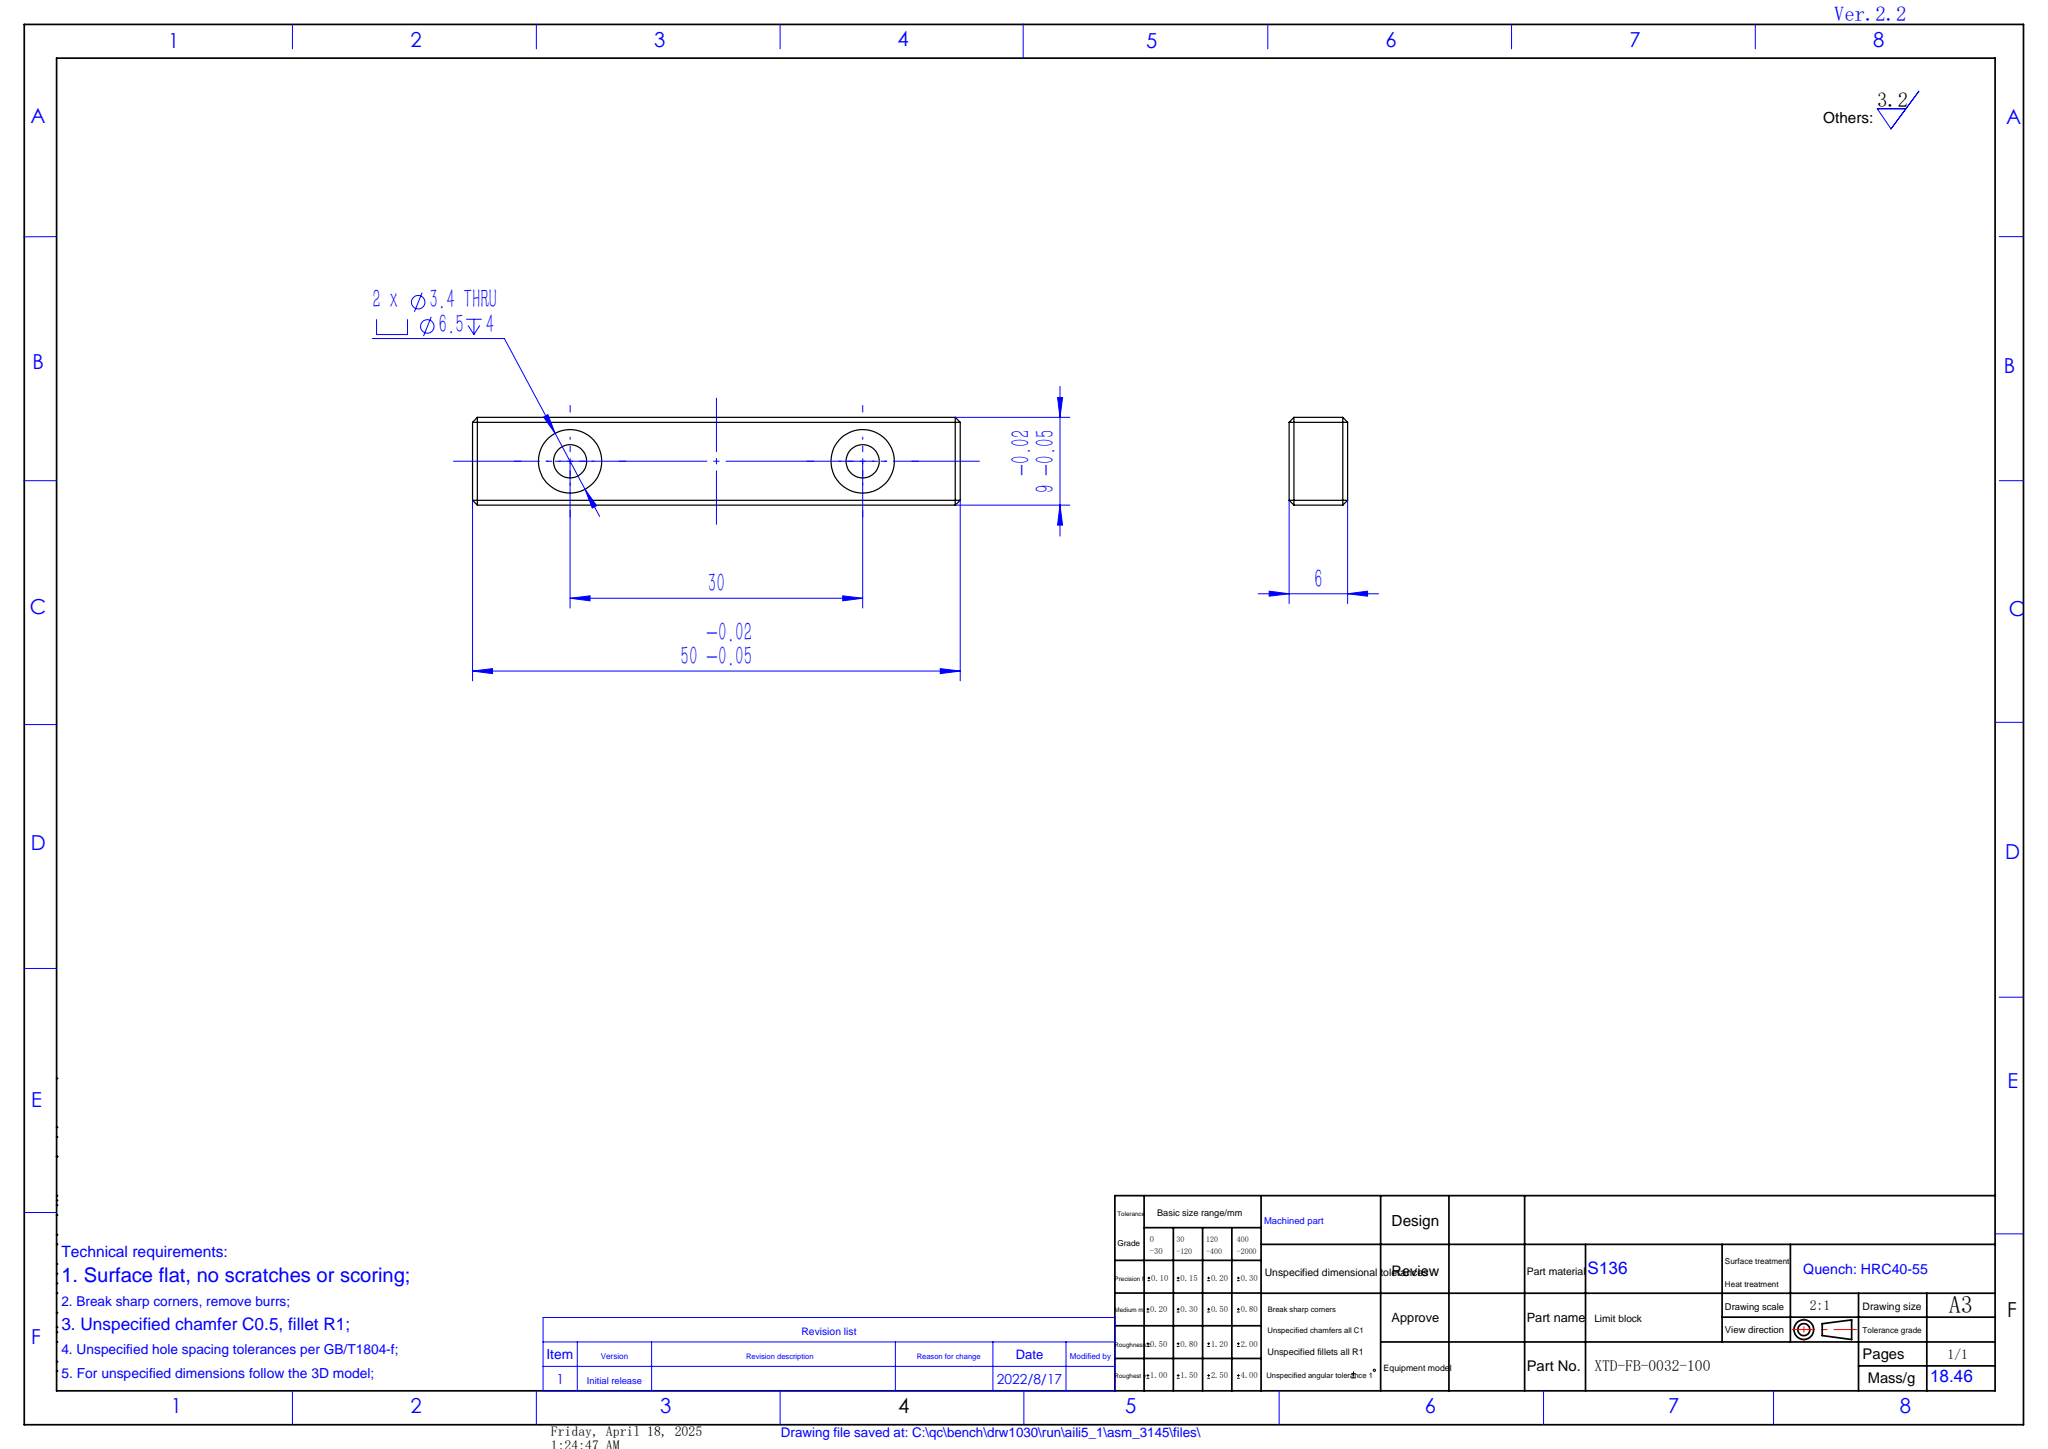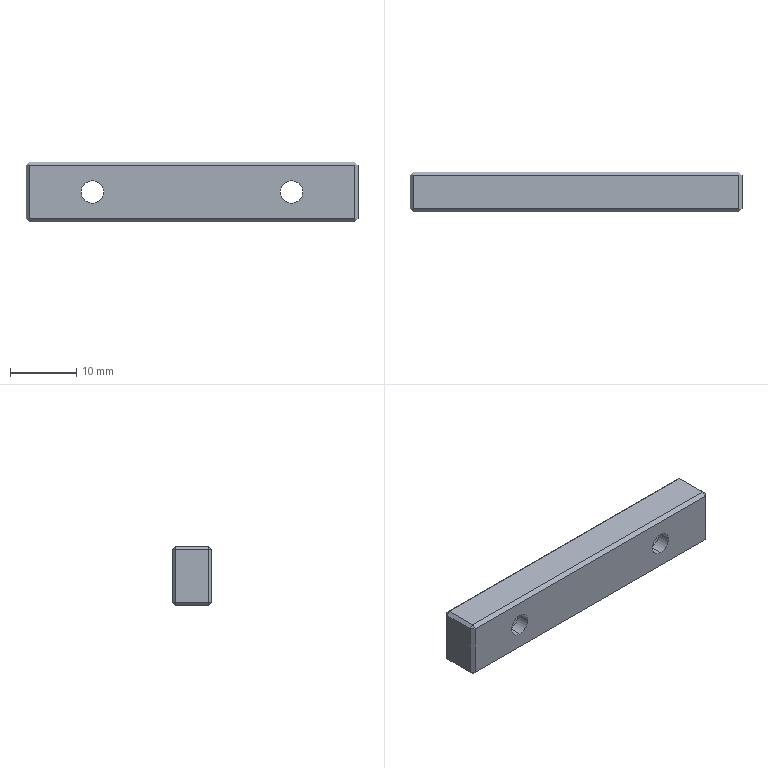Part | SolidWorks | features Chamfer 1, Extrusion 1, HoleWzd 1 | 1 solid | 36 faces | box 50 x 6 x 9 mm | volume 2366 mm3 | plane 28 | cylinder 8 | commonest cylinder face diameters 3.4 x4 6.5 x4
STEP:
#1=CARTESIAN_POINT('',(-15.,2.,-3.25));
#2=VERTEX_POINT('',#1);
#3=CARTESIAN_POINT('',(-15.,2.,3.25));
#4=VERTEX_POINT('',#3);
#5=CARTESIAN_POINT('',(-15.,2.,0.));
#6=DIRECTION('',(0.,1.,0.));
#7=DIRECTION('',(0.,0.,1.));
#8=AXIS2_PLACEMENT_3D('',#5,#6,#7);
#9=CIRCLE('',#8,3.25);
#10=EDGE_CURVE('',#2,#4,#9,.T.);
#11=ORIENTED_EDGE('',*,*,#10,.F.);
#12=CARTESIAN_POINT('',(-15.,6.,-3.25));
#13=VERTEX_POINT('',#12);
#14=CARTESIAN_POINT('',(-15.,6.,-3.25));
#15=DIRECTION('',(0.,1.,0.));
#16=VECTOR('',#15,1000.);
#17=LINE('',#14,#16);
#18=EDGE_CURVE('',#2,#13,#17,.T.);
#19=ORIENTED_EDGE('',*,*,#18,.T.);
#20=CARTESIAN_POINT('',(-15.,6.,3.25));
#21=VERTEX_POINT('',#20);
#22=CARTESIAN_POINT('',(-15.,6.,0.));
#23=DIRECTION('',(0.,1.,0.));
#24=DIRECTION('',(0.,0.,1.));
#25=AXIS2_PLACEMENT_3D('',#22,#23,#24);
#26=CIRCLE('',#25,3.25);
#27=EDGE_CURVE('',#13,#21,#26,.T.);
#28=ORIENTED_EDGE('',*,*,#27,.T.);
#29=CARTESIAN_POINT('',(-15.,6.,3.25));
#30=DIRECTION('',(0.,1.,0.));
#31=VECTOR('',#30,1000.);
#32=LINE('',#29,#31);
#33=EDGE_CURVE('',#4,#21,#32,.T.);
#34=ORIENTED_EDGE('',*,*,#33,.F.);
#35=EDGE_LOOP('',(#11,#19,#28,#34));
#36=FACE_OUTER_BOUND('',#35,.T.);
#37=CARTESIAN_POINT('',(-15.,6.,0.));
#38=DIRECTION('',(0.,1.,0.));
#39=DIRECTION('',(0.,0.,1.));
#40=AXIS2_PLACEMENT_3D('',#37,#38,#39);
#41=CYLINDRICAL_SURFACE('',#40,3.25);
#42=ADVANCED_FACE('',(#36),#41,.F.);
#43=CARTESIAN_POINT('',(-15.,0.,-1.7));
#44=VERTEX_POINT('',#43);
#45=CARTESIAN_POINT('',(-15.,0.,1.7));
#46=VERTEX_POINT('',#45);
#47=CARTESIAN_POINT('',(-15.,0.,0.));
#48=DIRECTION('',(0.,1.,0.));
#49=DIRECTION('',(0.,0.,1.));
#50=AXIS2_PLACEMENT_3D('',#47,#48,#49);
#51=CIRCLE('',#50,1.7);
#52=EDGE_CURVE('',#44,#46,#51,.T.);
#53=ORIENTED_EDGE('',*,*,#52,.F.);
#54=CARTESIAN_POINT('',(-15.,2.,-1.7));
#55=VERTEX_POINT('',#54);
#56=CARTESIAN_POINT('',(-15.,6.,-1.7));
#57=DIRECTION('',(0.,1.,0.));
#58=VECTOR('',#57,1000.);
#59=LINE('',#56,#58);
#60=EDGE_CURVE('',#44,#55,#59,.T.);
#61=ORIENTED_EDGE('',*,*,#60,.T.);
#62=CARTESIAN_POINT('',(-15.,2.,1.7));
#63=VERTEX_POINT('',#62);
#64=CARTESIAN_POINT('',(-15.,2.,0.));
#65=DIRECTION('',(0.,1.,0.));
#66=DIRECTION('',(0.,0.,1.));
#67=AXIS2_PLACEMENT_3D('',#64,#65,#66);
#68=CIRCLE('',#67,1.7);
#69=EDGE_CURVE('',#55,#63,#68,.T.);
#70=ORIENTED_EDGE('',*,*,#69,.T.);
#71=CARTESIAN_POINT('',(-15.,6.,1.7));
#72=DIRECTION('',(0.,1.,0.));
#73=VECTOR('',#72,1000.);
#74=LINE('',#71,#73);
#75=EDGE_CURVE('',#46,#63,#74,.T.);
#76=ORIENTED_EDGE('',*,*,#75,.F.);
#77=EDGE_LOOP('',(#53,#61,#70,#76));
#78=FACE_OUTER_BOUND('',#77,.T.);
#79=CARTESIAN_POINT('',(-15.,6.,0.));
#80=DIRECTION('',(0.,1.,0.));
#81=DIRECTION('',(0.,0.,1.));
#82=AXIS2_PLACEMENT_3D('',#79,#80,#81);
#83=CYLINDRICAL_SURFACE('',#82,1.7);
#84=ADVANCED_FACE('',(#78),#83,.F.);
#85=CARTESIAN_POINT('',(15.,2.,-3.25));
#86=VERTEX_POINT('',#85);
#87=CARTESIAN_POINT('',(15.,2.,3.25));
#88=VERTEX_POINT('',#87);
#89=CARTESIAN_POINT('',(15.,2.,0.));
#90=DIRECTION('',(0.,1.,0.));
#91=DIRECTION('',(0.,0.,1.));
#92=AXIS2_PLACEMENT_3D('',#89,#90,#91);
#93=CIRCLE('',#92,3.25);
#94=EDGE_CURVE('',#86,#88,#93,.T.);
#95=ORIENTED_EDGE('',*,*,#94,.F.);
#96=CARTESIAN_POINT('',(15.,6.,-3.25));
#97=VERTEX_POINT('',#96);
#98=CARTESIAN_POINT('',(15.,6.,-3.25));
#99=DIRECTION('',(0.,1.,0.));
#100=VECTOR('',#99,1000.);
#101=LINE('',#98,#100);
#102=EDGE_CURVE('',#86,#97,#101,.T.);
#103=ORIENTED_EDGE('',*,*,#102,.T.);
#104=CARTESIAN_POINT('',(15.,6.,3.25));
#105=VERTEX_POINT('',#104);
#106=CARTESIAN_POINT('',(15.,6.,0.));
#107=DIRECTION('',(0.,1.,0.));
#108=DIRECTION('',(0.,0.,1.));
#109=AXIS2_PLACEMENT_3D('',#106,#107,#108);
#110=CIRCLE('',#109,3.25);
#111=EDGE_CURVE('',#97,#105,#110,.T.);
#112=ORIENTED_EDGE('',*,*,#111,.T.);
#113=CARTESIAN_POINT('',(15.,6.,3.25));
#114=DIRECTION('',(0.,1.,0.));
#115=VECTOR('',#114,1000.);
#116=LINE('',#113,#115);
#117=EDGE_CURVE('',#88,#105,#116,.T.);
#118=ORIENTED_EDGE('',*,*,#117,.F.);
#119=EDGE_LOOP('',(#95,#103,#112,#118));
#120=FACE_OUTER_BOUND('',#119,.T.);
#121=CARTESIAN_POINT('',(15.,6.,0.));
#122=DIRECTION('',(0.,1.,0.));
#123=DIRECTION('',(0.,0.,1.));
#124=AXIS2_PLACEMENT_3D('',#121,#122,#123);
#125=CYLINDRICAL_SURFACE('',#124,3.25);
#126=ADVANCED_FACE('',(#120),#125,.F.);
#127=CARTESIAN_POINT('',(15.,0.,-1.7));
#128=VERTEX_POINT('',#127);
#129=CARTESIAN_POINT('',(15.,0.,1.7));
#130=VERTEX_POINT('',#129);
#131=CARTESIAN_POINT('',(15.,0.,0.));
#132=DIRECTION('',(0.,1.,0.));
#133=DIRECTION('',(0.,0.,1.));
#134=AXIS2_PLACEMENT_3D('',#131,#132,#133);
#135=CIRCLE('',#134,1.7);
#136=EDGE_CURVE('',#128,#130,#135,.T.);
#137=ORIENTED_EDGE('',*,*,#136,.F.);
#138=CARTESIAN_POINT('',(15.,2.,-1.7));
#139=VERTEX_POINT('',#138);
#140=CARTESIAN_POINT('',(15.,6.,-1.7));
#141=DIRECTION('',(0.,1.,0.));
#142=VECTOR('',#141,1000.);
#143=LINE('',#140,#142);
#144=EDGE_CURVE('',#128,#139,#143,.T.);
#145=ORIENTED_EDGE('',*,*,#144,.T.);
#146=CARTESIAN_POINT('',(15.,2.,1.7));
#147=VERTEX_POINT('',#146);
#148=CARTESIAN_POINT('',(15.,2.,0.));
#149=DIRECTION('',(0.,1.,0.));
#150=DIRECTION('',(0.,0.,1.));
#151=AXIS2_PLACEMENT_3D('',#148,#149,#150);
#152=CIRCLE('',#151,1.7);
#153=EDGE_CURVE('',#139,#147,#152,.T.);
#154=ORIENTED_EDGE('',*,*,#153,.T.);
#155=CARTESIAN_POINT('',(15.,6.,1.7));
#156=DIRECTION('',(0.,1.,0.));
#157=VECTOR('',#156,1000.);
#158=LINE('',#155,#157);
#159=EDGE_CURVE('',#130,#147,#158,.T.);
#160=ORIENTED_EDGE('',*,*,#159,.F.);
#161=EDGE_LOOP('',(#137,#145,#154,#160));
#162=FACE_OUTER_BOUND('',#161,.T.);
#163=CARTESIAN_POINT('',(15.,6.,0.));
#164=DIRECTION('',(0.,1.,0.));
#165=DIRECTION('',(0.,0.,1.));
#166=AXIS2_PLACEMENT_3D('',#163,#164,#165);
#167=CYLINDRICAL_SURFACE('',#166,1.7);
#168=ADVANCED_FACE('',(#162),#167,.F.);
#169=CARTESIAN_POINT('',(-25.,5.5,4.));
#170=VERTEX_POINT('',#169);
#171=CARTESIAN_POINT('',(-25.,5.5,-4.));
#172=VERTEX_POINT('',#171);
#173=CARTESIAN_POINT('',(-25.,5.5,-4.5));
#174=DIRECTION('',(0.,0.,-1.));
#175=VECTOR('',#174,1000.);
#176=LINE('',#173,#175);
#177=EDGE_CURVE('',#170,#172,#176,.T.);
#178=ORIENTED_EDGE('',*,*,#177,.T.);
#179=CARTESIAN_POINT('',(-25.,0.5,-4.));
#180=VERTEX_POINT('',#179);
#181=CARTESIAN_POINT('',(-25.,6.,-4.));
#182=DIRECTION('',(0.,-1.,0.));
#183=VECTOR('',#182,1000.);
#184=LINE('',#181,#183);
#185=EDGE_CURVE('',#172,#180,#184,.T.);
#186=ORIENTED_EDGE('',*,*,#185,.T.);
#187=CARTESIAN_POINT('',(-25.,0.5,4.));
#188=VERTEX_POINT('',#187);
#189=CARTESIAN_POINT('',(-25.,0.5,4.5));
#190=DIRECTION('',(0.,0.,1.));
#191=VECTOR('',#190,1000.);
#192=LINE('',#189,#191);
#193=EDGE_CURVE('',#180,#188,#192,.T.);
#194=ORIENTED_EDGE('',*,*,#193,.T.);
#195=CARTESIAN_POINT('',(-25.,6.,4.));
#196=DIRECTION('',(0.,1.,0.));
#197=VECTOR('',#196,1000.);
#198=LINE('',#195,#197);
#199=EDGE_CURVE('',#188,#170,#198,.T.);
#200=ORIENTED_EDGE('',*,*,#199,.T.);
#201=EDGE_LOOP('',(#178,#186,#194,#200));
#202=FACE_OUTER_BOUND('',#201,.T.);
#203=CARTESIAN_POINT('',(-25.,6.,4.5));
#204=DIRECTION('',(1.,0.,0.));
#205=DIRECTION('',(0.,0.,-1.));
#206=AXIS2_PLACEMENT_3D('',#203,#204,#205);
#207=PLANE('',#206);
#208=ADVANCED_FACE('',(#202),#207,.F.);
#209=CARTESIAN_POINT('',(-24.5,0.5,4.5));
#210=VERTEX_POINT('',#209);
#211=CARTESIAN_POINT('',(24.5,0.5,4.5));
#212=VERTEX_POINT('',#211);
#213=CARTESIAN_POINT('',(25.,0.5,4.5));
#214=DIRECTION('',(1.,0.,0.));
#215=VECTOR('',#214,1000.);
#216=LINE('',#213,#215);
#217=EDGE_CURVE('',#210,#212,#216,.T.);
#218=ORIENTED_EDGE('',*,*,#217,.T.);
#219=CARTESIAN_POINT('',(24.5,5.5,4.5));
#220=VERTEX_POINT('',#219);
#221=CARTESIAN_POINT('',(24.5,6.,4.5));
#222=DIRECTION('',(0.,1.,0.));
#223=VECTOR('',#222,1000.);
#224=LINE('',#221,#223);
#225=EDGE_CURVE('',#212,#220,#224,.T.);
#226=ORIENTED_EDGE('',*,*,#225,.T.);
#227=CARTESIAN_POINT('',(-24.5,5.5,4.5));
#228=VERTEX_POINT('',#227);
#229=CARTESIAN_POINT('',(-25.,5.5,4.5));
#230=DIRECTION('',(-1.,0.,0.));
#231=VECTOR('',#230,1000.);
#232=LINE('',#229,#231);
#233=EDGE_CURVE('',#220,#228,#232,.T.);
#234=ORIENTED_EDGE('',*,*,#233,.T.);
#235=CARTESIAN_POINT('',(-24.5,6.,4.5));
#236=DIRECTION('',(0.,-1.,0.));
#237=VECTOR('',#236,1000.);
#238=LINE('',#235,#237);
#239=EDGE_CURVE('',#228,#210,#238,.T.);
#240=ORIENTED_EDGE('',*,*,#239,.T.);
#241=EDGE_LOOP('',(#218,#226,#234,#240));
#242=FACE_OUTER_BOUND('',#241,.T.);
#243=CARTESIAN_POINT('',(25.,6.,4.5));
#244=DIRECTION('',(0.,0.,-1.));
#245=DIRECTION('',(-1.,0.,0.));
#246=AXIS2_PLACEMENT_3D('',#243,#244,#245);
#247=PLANE('',#246);
#248=ADVANCED_FACE('',(#242),#247,.F.);
#249=CARTESIAN_POINT('',(25.,5.5,4.));
#250=VERTEX_POINT('',#249);
#251=CARTESIAN_POINT('',(25.,0.5,4.));
#252=VERTEX_POINT('',#251);
#253=CARTESIAN_POINT('',(25.,6.,4.));
#254=DIRECTION('',(0.,-1.,0.));
#255=VECTOR('',#254,1000.);
#256=LINE('',#253,#255);
#257=EDGE_CURVE('',#250,#252,#256,.T.);
#258=ORIENTED_EDGE('',*,*,#257,.T.);
#259=CARTESIAN_POINT('',(25.,0.5,-4.));
#260=VERTEX_POINT('',#259);
#261=CARTESIAN_POINT('',(25.,0.5,4.5));
#262=DIRECTION('',(0.,0.,-1.));
#263=VECTOR('',#262,1000.);
#264=LINE('',#261,#263);
#265=EDGE_CURVE('',#252,#260,#264,.T.);
#266=ORIENTED_EDGE('',*,*,#265,.T.);
#267=CARTESIAN_POINT('',(25.,5.5,-4.));
#268=VERTEX_POINT('',#267);
#269=CARTESIAN_POINT('',(25.,6.,-4.));
#270=DIRECTION('',(0.,1.,0.));
#271=VECTOR('',#270,1000.);
#272=LINE('',#269,#271);
#273=EDGE_CURVE('',#260,#268,#272,.T.);
#274=ORIENTED_EDGE('',*,*,#273,.T.);
#275=CARTESIAN_POINT('',(25.,5.5,4.5));
#276=DIRECTION('',(0.,0.,1.));
#277=VECTOR('',#276,1000.);
#278=LINE('',#275,#277);
#279=EDGE_CURVE('',#268,#250,#278,.T.);
#280=ORIENTED_EDGE('',*,*,#279,.T.);
#281=EDGE_LOOP('',(#258,#266,#274,#280));
#282=FACE_OUTER_BOUND('',#281,.T.);
#283=CARTESIAN_POINT('',(25.,6.,4.5));
#284=DIRECTION('',(-1.,0.,0.));
#285=DIRECTION('',(0.,0.,1.));
#286=AXIS2_PLACEMENT_3D('',#283,#284,#285);
#287=PLANE('',#286);
#288=ADVANCED_FACE('',(#282),#287,.F.);
#289=CARTESIAN_POINT('',(24.5,5.5,-4.5));
#290=VERTEX_POINT('',#289);
#291=CARTESIAN_POINT('',(24.5,0.5,-4.5));
#292=VERTEX_POINT('',#291);
#293=CARTESIAN_POINT('',(24.5,6.,-4.5));
#294=DIRECTION('',(0.,-1.,0.));
#295=VECTOR('',#294,1000.);
#296=LINE('',#293,#295);
#297=EDGE_CURVE('',#290,#292,#296,.T.);
#298=ORIENTED_EDGE('',*,*,#297,.T.);
#299=CARTESIAN_POINT('',(-24.5,0.5,-4.5));
#300=VERTEX_POINT('',#299);
#301=CARTESIAN_POINT('',(25.,0.5,-4.5));
#302=DIRECTION('',(-1.,0.,0.));
#303=VECTOR('',#302,1000.);
#304=LINE('',#301,#303);
#305=EDGE_CURVE('',#292,#300,#304,.T.);
#306=ORIENTED_EDGE('',*,*,#305,.T.);
#307=CARTESIAN_POINT('',(-24.5,5.5,-4.5));
#308=VERTEX_POINT('',#307);
#309=CARTESIAN_POINT('',(-24.5,6.,-4.5));
#310=DIRECTION('',(0.,1.,0.));
#311=VECTOR('',#310,1000.);
#312=LINE('',#309,#311);
#313=EDGE_CURVE('',#300,#308,#312,.T.);
#314=ORIENTED_EDGE('',*,*,#313,.T.);
#315=CARTESIAN_POINT('',(25.,5.5,-4.5));
#316=DIRECTION('',(1.,0.,0.));
#317=VECTOR('',#316,1000.);
#318=LINE('',#315,#317);
#319=EDGE_CURVE('',#308,#290,#318,.T.);
#320=ORIENTED_EDGE('',*,*,#319,.T.);
#321=EDGE_LOOP('',(#298,#306,#314,#320));
#322=FACE_OUTER_BOUND('',#321,.T.);
#323=CARTESIAN_POINT('',(25.,6.,-4.5));
#324=DIRECTION('',(0.,0.,1.));
#325=DIRECTION('',(1.,0.,0.));
#326=AXIS2_PLACEMENT_3D('',#323,#324,#325);
#327=PLANE('',#326);
#328=ADVANCED_FACE('',(#322),#327,.F.);
#329=CARTESIAN_POINT('',(-15.,6.,0.));
#330=DIRECTION('',(0.,1.,0.));
#331=DIRECTION('',(0.,0.,1.));
#332=AXIS2_PLACEMENT_3D('',#329,#330,#331);
#333=CIRCLE('',#332,3.25);
#334=EDGE_CURVE('',#21,#13,#333,.T.);
#335=ORIENTED_EDGE('',*,*,#334,.F.);
#336=ORIENTED_EDGE('',*,*,#27,.F.);
#337=EDGE_LOOP('',(#335,#336));
#338=FACE_BOUND('',#337,.T.);
#339=CARTESIAN_POINT('',(15.,6.,0.));
#340=DIRECTION('',(0.,1.,0.));
#341=DIRECTION('',(0.,0.,1.));
#342=AXIS2_PLACEMENT_3D('',#339,#340,#341);
#343=CIRCLE('',#342,3.25);
#344=EDGE_CURVE('',#105,#97,#343,.T.);
#345=ORIENTED_EDGE('',*,*,#344,.F.);
#346=ORIENTED_EDGE('',*,*,#111,.F.);
#347=EDGE_LOOP('',(#345,#346));
#348=FACE_BOUND('',#347,.T.);
#349=CARTESIAN_POINT('',(24.5,6.,4.));
#350=VERTEX_POINT('',#349);
#351=CARTESIAN_POINT('',(24.5,6.,-4.));
#352=VERTEX_POINT('',#351);
#353=CARTESIAN_POINT('',(24.5,6.,-4.5));
#354=DIRECTION('',(0.,0.,-1.));
#355=VECTOR('',#354,1000.);
#356=LINE('',#353,#355);
#357=EDGE_CURVE('',#350,#352,#356,.T.);
#358=ORIENTED_EDGE('',*,*,#357,.T.);
#359=CARTESIAN_POINT('',(-24.5,6.,-4.));
#360=VERTEX_POINT('',#359);
#361=CARTESIAN_POINT('',(-25.,6.,-4.));
#362=DIRECTION('',(-1.,0.,0.));
#363=VECTOR('',#362,1000.);
#364=LINE('',#361,#363);
#365=EDGE_CURVE('',#352,#360,#364,.T.);
#366=ORIENTED_EDGE('',*,*,#365,.T.);
#367=CARTESIAN_POINT('',(-24.5,6.,4.));
#368=VERTEX_POINT('',#367);
#369=CARTESIAN_POINT('',(-24.5,6.,4.5));
#370=DIRECTION('',(0.,0.,1.));
#371=VECTOR('',#370,1000.);
#372=LINE('',#369,#371);
#373=EDGE_CURVE('',#360,#368,#372,.T.);
#374=ORIENTED_EDGE('',*,*,#373,.T.);
#375=CARTESIAN_POINT('',(25.,6.,4.));
#376=DIRECTION('',(1.,0.,0.));
#377=VECTOR('',#376,1000.);
#378=LINE('',#375,#377);
#379=EDGE_CURVE('',#368,#350,#378,.T.);
#380=ORIENTED_EDGE('',*,*,#379,.T.);
#381=EDGE_LOOP('',(#358,#366,#374,#380));
#382=FACE_OUTER_BOUND('',#381,.T.);
#383=CARTESIAN_POINT('',(0.,6.,0.));
#384=DIRECTION('',(0.,1.,0.));
#385=DIRECTION('',(0.,0.,1.));
#386=AXIS2_PLACEMENT_3D('',#383,#384,#385);
#387=PLANE('',#386);
#388=ADVANCED_FACE('',(#338,#348,#382),#387,.T.);
#389=CARTESIAN_POINT('',(-15.,0.,0.));
#390=DIRECTION('',(0.,1.,0.));
#391=DIRECTION('',(0.,0.,1.));
#392=AXIS2_PLACEMENT_3D('',#389,#390,#391);
#393=CIRCLE('',#392,1.7);
#394=EDGE_CURVE('',#46,#44,#393,.T.);
#395=ORIENTED_EDGE('',*,*,#394,.T.);
#396=ORIENTED_EDGE('',*,*,#52,.T.);
#397=EDGE_LOOP('',(#395,#396));
#398=FACE_BOUND('',#397,.T.);
#399=CARTESIAN_POINT('',(15.,0.,0.));
#400=DIRECTION('',(0.,1.,0.));
#401=DIRECTION('',(0.,0.,1.));
#402=AXIS2_PLACEMENT_3D('',#399,#400,#401);
#403=CIRCLE('',#402,1.7);
#404=EDGE_CURVE('',#130,#128,#403,.T.);
#405=ORIENTED_EDGE('',*,*,#404,.T.);
#406=ORIENTED_EDGE('',*,*,#136,.T.);
#407=EDGE_LOOP('',(#405,#406));
#408=FACE_BOUND('',#407,.T.);
#409=CARTESIAN_POINT('',(24.5,0.,-4.));
#410=VERTEX_POINT('',#409);
#411=CARTESIAN_POINT('',(24.5,0.,4.));
#412=VERTEX_POINT('',#411);
#413=CARTESIAN_POINT('',(24.5,0.,0.));
#414=DIRECTION('',(0.,0.,1.));
#415=VECTOR('',#414,1000.);
#416=LINE('',#413,#415);
#417=EDGE_CURVE('',#410,#412,#416,.T.);
#418=ORIENTED_EDGE('',*,*,#417,.T.);
#419=CARTESIAN_POINT('',(-24.5,0.,4.));
#420=VERTEX_POINT('',#419);
#421=CARTESIAN_POINT('',(0.,0.,4.));
#422=DIRECTION('',(-1.,0.,0.));
#423=VECTOR('',#422,1000.);
#424=LINE('',#421,#423);
#425=EDGE_CURVE('',#412,#420,#424,.T.);
#426=ORIENTED_EDGE('',*,*,#425,.T.);
#427=CARTESIAN_POINT('',(-24.5,0.,-4.));
#428=VERTEX_POINT('',#427);
#429=CARTESIAN_POINT('',(-24.5,0.,0.));
#430=DIRECTION('',(0.,0.,-1.));
#431=VECTOR('',#430,1000.);
#432=LINE('',#429,#431);
#433=EDGE_CURVE('',#420,#428,#432,.T.);
#434=ORIENTED_EDGE('',*,*,#433,.T.);
#435=CARTESIAN_POINT('',(0.,0.,-4.));
#436=DIRECTION('',(1.,0.,0.));
#437=VECTOR('',#436,1000.);
#438=LINE('',#435,#437);
#439=EDGE_CURVE('',#428,#410,#438,.T.);
#440=ORIENTED_EDGE('',*,*,#439,.T.);
#441=EDGE_LOOP('',(#418,#426,#434,#440));
#442=FACE_OUTER_BOUND('',#441,.T.);
#443=CARTESIAN_POINT('',(0.,0.,0.));
#444=DIRECTION('',(0.,1.,0.));
#445=DIRECTION('',(0.,0.,1.));
#446=AXIS2_PLACEMENT_3D('',#443,#444,#445);
#447=PLANE('',#446);
#448=ADVANCED_FACE('',(#398,#408,#442),#447,.F.);
#449=CARTESIAN_POINT('',(-24.5,5.5,-4.5));
#450=DIRECTION('',(-0.7071,0.,0.7071));
#451=VECTOR('',#450,1000.);
#452=LINE('',#449,#451);
#453=EDGE_CURVE('',#308,#172,#452,.T.);
#454=ORIENTED_EDGE('',*,*,#453,.F.);
#455=ORIENTED_EDGE('',*,*,#313,.F.);
#456=CARTESIAN_POINT('',(-25.,0.5,-4.));
#457=DIRECTION('',(0.7071,0.,-0.7071));
#458=VECTOR('',#457,1000.);
#459=LINE('',#456,#458);
#460=EDGE_CURVE('',#180,#300,#459,.T.);
#461=ORIENTED_EDGE('',*,*,#460,.F.);
#462=ORIENTED_EDGE('',*,*,#185,.F.);
#463=EDGE_LOOP('',(#454,#455,#461,#462));
#464=FACE_OUTER_BOUND('',#463,.T.);
#465=CARTESIAN_POINT('',(-25.,6.,-4.));
#466=DIRECTION('',(0.7071,0.,0.7071));
#467=DIRECTION('',(0.,-1.,0.));
#468=AXIS2_PLACEMENT_3D('',#465,#466,#467);
#469=PLANE('',#468);
#470=ADVANCED_FACE('',(#464),#469,.F.);
#471=CARTESIAN_POINT('',(-24.5,5.5,-4.5));
#472=DIRECTION('',(0.,0.7071,0.7071));
#473=VECTOR('',#472,1000.);
#474=LINE('',#471,#473);
#475=EDGE_CURVE('',#308,#360,#474,.T.);
#476=ORIENTED_EDGE('',*,*,#475,.F.);
#477=ORIENTED_EDGE('',*,*,#453,.T.);
#478=CARTESIAN_POINT('',(-24.75,5.75,-4.));
#479=DIRECTION('',(-0.7071,-0.7071,0.));
#480=VECTOR('',#479,1000.);
#481=LINE('',#478,#480);
#482=EDGE_CURVE('',#360,#172,#481,.T.);
#483=ORIENTED_EDGE('',*,*,#482,.F.);
#484=EDGE_LOOP('',(#476,#477,#483));
#485=FACE_OUTER_BOUND('',#484,.T.);
#486=CARTESIAN_POINT('',(-24.5,5.5,-4.5));
#487=DIRECTION('',(-0.5774,0.5774,-0.5774));
#488=DIRECTION('',(-0.7071,0.,0.7071));
#489=AXIS2_PLACEMENT_3D('',#486,#487,#488);
#490=PLANE('',#489);
#491=ADVANCED_FACE('',(#485),#490,.T.);
#492=CARTESIAN_POINT('',(-25.,0.5,-4.));
#493=DIRECTION('',(0.7071,-0.7071,0.));
#494=VECTOR('',#493,1000.);
#495=LINE('',#492,#494);
#496=EDGE_CURVE('',#180,#428,#495,.T.);
#497=ORIENTED_EDGE('',*,*,#496,.F.);
#498=ORIENTED_EDGE('',*,*,#460,.T.);
#499=CARTESIAN_POINT('',(-24.5,0.25,-4.25));
#500=DIRECTION('',(0.,0.7071,-0.7071));
#501=VECTOR('',#500,1000.);
#502=LINE('',#499,#501);
#503=EDGE_CURVE('',#428,#300,#502,.T.);
#504=ORIENTED_EDGE('',*,*,#503,.F.);
#505=EDGE_LOOP('',(#497,#498,#504));
#506=FACE_OUTER_BOUND('',#505,.T.);
#507=CARTESIAN_POINT('',(-25.,0.5,-4.));
#508=DIRECTION('',(-0.5774,-0.5774,-0.5774));
#509=DIRECTION('',(0.7071,-0.7071,0.));
#510=AXIS2_PLACEMENT_3D('',#507,#508,#509);
#511=PLANE('',#510);
#512=ADVANCED_FACE('',(#506),#511,.T.);
#513=ORIENTED_EDGE('',*,*,#482,.T.);
#514=ORIENTED_EDGE('',*,*,#177,.F.);
#515=CARTESIAN_POINT('',(-25.,5.5,4.));
#516=DIRECTION('',(-0.7071,-0.7071,0.));
#517=VECTOR('',#516,1000.);
#518=LINE('',#515,#517);
#519=EDGE_CURVE('',#368,#170,#518,.T.);
#520=ORIENTED_EDGE('',*,*,#519,.F.);
#521=ORIENTED_EDGE('',*,*,#373,.F.);
#522=EDGE_LOOP('',(#513,#514,#520,#521));
#523=FACE_OUTER_BOUND('',#522,.T.);
#524=CARTESIAN_POINT('',(-24.5,6.,0.));
#525=DIRECTION('',(-0.7071,0.7071,0.));
#526=DIRECTION('',(0.,0.,-1.));
#527=AXIS2_PLACEMENT_3D('',#524,#525,#526);
#528=PLANE('',#527);
#529=ADVANCED_FACE('',(#523),#528,.T.);
#530=ORIENTED_EDGE('',*,*,#475,.T.);
#531=ORIENTED_EDGE('',*,*,#365,.F.);
#532=CARTESIAN_POINT('',(24.5,5.75,-4.25));
#533=DIRECTION('',(0.,0.7071,0.7071));
#534=VECTOR('',#533,1000.);
#535=LINE('',#532,#534);
#536=EDGE_CURVE('',#290,#352,#535,.T.);
#537=ORIENTED_EDGE('',*,*,#536,.F.);
#538=ORIENTED_EDGE('',*,*,#319,.F.);
#539=EDGE_LOOP('',(#530,#531,#537,#538));
#540=FACE_OUTER_BOUND('',#539,.T.);
#541=CARTESIAN_POINT('',(0.,6.,-4.));
#542=DIRECTION('',(0.,0.7071,-0.7071));
#543=DIRECTION('',(1.,0.,0.));
#544=AXIS2_PLACEMENT_3D('',#541,#542,#543);
#545=PLANE('',#544);
#546=ADVANCED_FACE('',(#540),#545,.T.);
#547=CARTESIAN_POINT('',(24.5,0.5,-4.5));
#548=DIRECTION('',(0.7071,0.,0.7071));
#549=VECTOR('',#548,1000.);
#550=LINE('',#547,#549);
#551=EDGE_CURVE('',#292,#260,#550,.T.);
#552=ORIENTED_EDGE('',*,*,#551,.F.);
#553=ORIENTED_EDGE('',*,*,#297,.F.);
#554=CARTESIAN_POINT('',(25.,5.5,-4.));
#555=DIRECTION('',(-0.7071,0.,-0.7071));
#556=VECTOR('',#555,1000.);
#557=LINE('',#554,#556);
#558=EDGE_CURVE('',#268,#290,#557,.T.);
#559=ORIENTED_EDGE('',*,*,#558,.F.);
#560=ORIENTED_EDGE('',*,*,#273,.F.);
#561=EDGE_LOOP('',(#552,#553,#559,#560));
#562=FACE_OUTER_BOUND('',#561,.T.);
#563=CARTESIAN_POINT('',(24.5,6.,-4.5));
#564=DIRECTION('',(-0.7071,0.,0.7071));
#565=DIRECTION('',(0.,-1.,0.));
#566=AXIS2_PLACEMENT_3D('',#563,#564,#565);
#567=PLANE('',#566);
#568=ADVANCED_FACE('',(#562),#567,.F.);
#569=ORIENTED_EDGE('',*,*,#503,.T.);
#570=ORIENTED_EDGE('',*,*,#305,.F.);
#571=CARTESIAN_POINT('',(24.5,0.5,-4.5));
#572=DIRECTION('',(0.,0.7071,-0.7071));
#573=VECTOR('',#572,1000.);
#574=LINE('',#571,#573);
#575=EDGE_CURVE('',#410,#292,#574,.T.);
#576=ORIENTED_EDGE('',*,*,#575,.F.);
#577=ORIENTED_EDGE('',*,*,#439,.F.);
#578=EDGE_LOOP('',(#569,#570,#576,#577));
#579=FACE_OUTER_BOUND('',#578,.T.);
#580=CARTESIAN_POINT('',(25.,0.5,-4.5));
#581=DIRECTION('',(0.,0.7071,0.7071));
#582=DIRECTION('',(-1.,0.,0.));
#583=AXIS2_PLACEMENT_3D('',#580,#581,#582);
#584=PLANE('',#583);
#585=ADVANCED_FACE('',(#579),#584,.F.);
#586=ORIENTED_EDGE('',*,*,#496,.T.);
#587=ORIENTED_EDGE('',*,*,#433,.F.);
#588=CARTESIAN_POINT('',(-24.5,0.,4.));
#589=DIRECTION('',(0.7071,-0.7071,0.));
#590=VECTOR('',#589,1000.);
#591=LINE('',#588,#590);
#592=EDGE_CURVE('',#188,#420,#591,.T.);
#593=ORIENTED_EDGE('',*,*,#592,.F.);
#594=ORIENTED_EDGE('',*,*,#193,.F.);
#595=EDGE_LOOP('',(#586,#587,#593,#594));
#596=FACE_OUTER_BOUND('',#595,.T.);
#597=CARTESIAN_POINT('',(-25.,0.5,4.5));
#598=DIRECTION('',(0.7071,0.7071,0.));
#599=DIRECTION('',(0.,0.,1.));
#600=AXIS2_PLACEMENT_3D('',#597,#598,#599);
#601=PLANE('',#600);
#602=ADVANCED_FACE('',(#596),#601,.F.);
#603=CARTESIAN_POINT('',(-25.,5.5,4.));
#604=DIRECTION('',(0.7071,0.,0.7071));
#605=VECTOR('',#604,1000.);
#606=LINE('',#603,#605);
#607=EDGE_CURVE('',#170,#228,#606,.T.);
#608=ORIENTED_EDGE('',*,*,#607,.F.);
#609=ORIENTED_EDGE('',*,*,#199,.F.);
#610=CARTESIAN_POINT('',(-24.75,0.5,4.25));
#611=DIRECTION('',(-0.7071,0.,-0.7071));
#612=VECTOR('',#611,1000.);
#613=LINE('',#610,#612);
#614=EDGE_CURVE('',#210,#188,#613,.T.);
#615=ORIENTED_EDGE('',*,*,#614,.F.);
#616=ORIENTED_EDGE('',*,*,#239,.F.);
#617=EDGE_LOOP('',(#608,#609,#615,#616));
#618=FACE_OUTER_BOUND('',#617,.T.);
#619=CARTESIAN_POINT('',(-24.5,6.,4.5));
#620=DIRECTION('',(0.7071,0.,-0.7071));
#621=DIRECTION('',(0.,-1.,0.));
#622=AXIS2_PLACEMENT_3D('',#619,#620,#621);
#623=PLANE('',#622);
#624=ADVANCED_FACE('',(#618),#623,.F.);
#625=ORIENTED_EDGE('',*,*,#519,.T.);
#626=ORIENTED_EDGE('',*,*,#607,.T.);
#627=CARTESIAN_POINT('',(-24.5,5.75,4.25));
#628=DIRECTION('',(0.,-0.7071,0.7071));
#629=VECTOR('',#628,1000.);
#630=LINE('',#627,#629);
#631=EDGE_CURVE('',#368,#228,#630,.T.);
#632=ORIENTED_EDGE('',*,*,#631,.F.);
#633=EDGE_LOOP('',(#625,#626,#632));
#634=FACE_OUTER_BOUND('',#633,.T.);
#635=CARTESIAN_POINT('',(-25.,5.5,4.));
#636=DIRECTION('',(-0.5774,0.5774,0.5774));
#637=DIRECTION('',(0.7071,0.,0.7071));
#638=AXIS2_PLACEMENT_3D('',#635,#636,#637);
#639=PLANE('',#638);
#640=ADVANCED_FACE('',(#634),#639,.T.);
#641=ORIENTED_EDGE('',*,*,#558,.T.);
#642=ORIENTED_EDGE('',*,*,#536,.T.);
#643=CARTESIAN_POINT('',(25.,5.5,-4.));
#644=DIRECTION('',(-0.7071,0.7071,0.));
#645=VECTOR('',#644,1000.);
#646=LINE('',#643,#645);
#647=EDGE_CURVE('',#268,#352,#646,.T.);
#648=ORIENTED_EDGE('',*,*,#647,.F.);
#649=EDGE_LOOP('',(#641,#642,#648));
#650=FACE_OUTER_BOUND('',#649,.T.);
#651=CARTESIAN_POINT('',(25.,5.5,-4.));
#652=DIRECTION('',(0.5774,0.5774,-0.5774));
#653=DIRECTION('',(-0.7071,0.,-0.7071));
#654=AXIS2_PLACEMENT_3D('',#651,#652,#653);
#655=PLANE('',#654);
#656=ADVANCED_FACE('',(#650),#655,.T.);
#657=ORIENTED_EDGE('',*,*,#575,.T.);
#658=ORIENTED_EDGE('',*,*,#551,.T.);
#659=CARTESIAN_POINT('',(24.75,0.25,-4.));
#660=DIRECTION('',(0.7071,0.7071,0.));
#661=VECTOR('',#660,1000.);
#662=LINE('',#659,#661);
#663=EDGE_CURVE('',#410,#260,#662,.T.);
#664=ORIENTED_EDGE('',*,*,#663,.F.);
#665=EDGE_LOOP('',(#657,#658,#664));
#666=FACE_OUTER_BOUND('',#665,.T.);
#667=CARTESIAN_POINT('',(24.5,0.5,-4.5));
#668=DIRECTION('',(0.5774,-0.5774,-0.5774));
#669=DIRECTION('',(0.7071,0.7071,0.));
#670=AXIS2_PLACEMENT_3D('',#667,#668,#669);
#671=PLANE('',#670);
#672=ADVANCED_FACE('',(#666),#671,.T.);
#673=ORIENTED_EDGE('',*,*,#614,.T.);
#674=ORIENTED_EDGE('',*,*,#592,.T.);
#675=CARTESIAN_POINT('',(-24.5,0.,4.));
#676=DIRECTION('',(0.,-0.7071,-0.7071));
#677=VECTOR('',#676,1000.);
#678=LINE('',#675,#677);
#679=EDGE_CURVE('',#210,#420,#678,.T.);
#680=ORIENTED_EDGE('',*,*,#679,.F.);
#681=EDGE_LOOP('',(#673,#674,#680));
#682=FACE_OUTER_BOUND('',#681,.T.);
#683=CARTESIAN_POINT('',(-24.5,0.,4.));
#684=DIRECTION('',(-0.5774,-0.5774,0.5774));
#685=DIRECTION('',(0.7071,-0.7071,0.));
#686=AXIS2_PLACEMENT_3D('',#683,#684,#685);
#687=PLANE('',#686);
#688=ADVANCED_FACE('',(#682),#687,.T.);
#689=ORIENTED_EDGE('',*,*,#631,.T.);
#690=ORIENTED_EDGE('',*,*,#233,.F.);
#691=CARTESIAN_POINT('',(24.5,5.5,4.5));
#692=DIRECTION('',(0.,-0.7071,0.7071));
#693=VECTOR('',#692,1000.);
#694=LINE('',#691,#693);
#695=EDGE_CURVE('',#350,#220,#694,.T.);
#696=ORIENTED_EDGE('',*,*,#695,.F.);
#697=ORIENTED_EDGE('',*,*,#379,.F.);
#698=EDGE_LOOP('',(#689,#690,#696,#697));
#699=FACE_OUTER_BOUND('',#698,.T.);
#700=CARTESIAN_POINT('',(0.,6.,4.));
#701=DIRECTION('',(0.,0.7071,0.7071));
#702=DIRECTION('',(-1.,0.,0.));
#703=AXIS2_PLACEMENT_3D('',#700,#701,#702);
#704=PLANE('',#703);
#705=ADVANCED_FACE('',(#699),#704,.T.);
#706=ORIENTED_EDGE('',*,*,#647,.T.);
#707=ORIENTED_EDGE('',*,*,#357,.F.);
#708=CARTESIAN_POINT('',(24.75,5.75,4.));
#709=DIRECTION('',(-0.7071,0.7071,0.));
#710=VECTOR('',#709,1000.);
#711=LINE('',#708,#710);
#712=EDGE_CURVE('',#250,#350,#711,.T.);
#713=ORIENTED_EDGE('',*,*,#712,.F.);
#714=ORIENTED_EDGE('',*,*,#279,.F.);
#715=EDGE_LOOP('',(#706,#707,#713,#714));
#716=FACE_OUTER_BOUND('',#715,.T.);
#717=CARTESIAN_POINT('',(24.5,6.,0.));
#718=DIRECTION('',(0.7071,0.7071,0.));
#719=DIRECTION('',(0.,0.,1.));
#720=AXIS2_PLACEMENT_3D('',#717,#718,#719);
#721=PLANE('',#720);
#722=ADVANCED_FACE('',(#716),#721,.T.);
#723=ORIENTED_EDGE('',*,*,#663,.T.);
#724=ORIENTED_EDGE('',*,*,#265,.F.);
#725=CARTESIAN_POINT('',(25.,0.5,4.));
#726=DIRECTION('',(0.7071,0.7071,0.));
#727=VECTOR('',#726,1000.);
#728=LINE('',#725,#727);
#729=EDGE_CURVE('',#412,#252,#728,.T.);
#730=ORIENTED_EDGE('',*,*,#729,.F.);
#731=ORIENTED_EDGE('',*,*,#417,.F.);
#732=EDGE_LOOP('',(#723,#724,#730,#731));
#733=FACE_OUTER_BOUND('',#732,.T.);
#734=CARTESIAN_POINT('',(25.,0.5,4.5));
#735=DIRECTION('',(-0.7071,0.7071,0.));
#736=DIRECTION('',(0.,0.,-1.));
#737=AXIS2_PLACEMENT_3D('',#734,#735,#736);
#738=PLANE('',#737);
#739=ADVANCED_FACE('',(#733),#738,.F.);
#740=ORIENTED_EDGE('',*,*,#679,.T.);
#741=ORIENTED_EDGE('',*,*,#425,.F.);
#742=CARTESIAN_POINT('',(24.5,0.25,4.25));
#743=DIRECTION('',(0.,-0.7071,-0.7071));
#744=VECTOR('',#743,1000.);
#745=LINE('',#742,#744);
#746=EDGE_CURVE('',#212,#412,#745,.T.);
#747=ORIENTED_EDGE('',*,*,#746,.F.);
#748=ORIENTED_EDGE('',*,*,#217,.F.);
#749=EDGE_LOOP('',(#740,#741,#747,#748));
#750=FACE_OUTER_BOUND('',#749,.T.);
#751=CARTESIAN_POINT('',(25.,0.5,4.5));
#752=DIRECTION('',(0.,0.7071,-0.7071));
#753=DIRECTION('',(1.,0.,0.));
#754=AXIS2_PLACEMENT_3D('',#751,#752,#753);
#755=PLANE('',#754);
#756=ADVANCED_FACE('',(#750),#755,.F.);
#757=ORIENTED_EDGE('',*,*,#712,.T.);
#758=ORIENTED_EDGE('',*,*,#695,.T.);
#759=CARTESIAN_POINT('',(24.5,5.5,4.5));
#760=DIRECTION('',(-0.7071,0.,0.7071));
#761=VECTOR('',#760,1000.);
#762=LINE('',#759,#761);
#763=EDGE_CURVE('',#250,#220,#762,.T.);
#764=ORIENTED_EDGE('',*,*,#763,.F.);
#765=EDGE_LOOP('',(#757,#758,#764));
#766=FACE_OUTER_BOUND('',#765,.T.);
#767=CARTESIAN_POINT('',(24.5,5.5,4.5));
#768=DIRECTION('',(0.5774,0.5774,0.5774));
#769=DIRECTION('',(0.7071,0.,-0.7071));
#770=AXIS2_PLACEMENT_3D('',#767,#768,#769);
#771=PLANE('',#770);
#772=ADVANCED_FACE('',(#766),#771,.T.);
#773=ORIENTED_EDGE('',*,*,#746,.T.);
#774=ORIENTED_EDGE('',*,*,#729,.T.);
#775=CARTESIAN_POINT('',(25.,0.5,4.));
#776=DIRECTION('',(0.7071,0.,-0.7071));
#777=VECTOR('',#776,1000.);
#778=LINE('',#775,#777);
#779=EDGE_CURVE('',#212,#252,#778,.T.);
#780=ORIENTED_EDGE('',*,*,#779,.F.);
#781=EDGE_LOOP('',(#773,#774,#780));
#782=FACE_OUTER_BOUND('',#781,.T.);
#783=CARTESIAN_POINT('',(25.,0.5,4.));
#784=DIRECTION('',(0.5774,-0.5774,0.5774));
#785=DIRECTION('',(0.,-0.7071,-0.7071));
#786=AXIS2_PLACEMENT_3D('',#783,#784,#785);
#787=PLANE('',#786);
#788=ADVANCED_FACE('',(#782),#787,.T.);
#789=ORIENTED_EDGE('',*,*,#763,.T.);
#790=ORIENTED_EDGE('',*,*,#225,.F.);
#791=ORIENTED_EDGE('',*,*,#779,.T.);
#792=ORIENTED_EDGE('',*,*,#257,.F.);
#793=EDGE_LOOP('',(#789,#790,#791,#792));
#794=FACE_OUTER_BOUND('',#793,.T.);
#795=CARTESIAN_POINT('',(25.,6.,4.));
#796=DIRECTION('',(-0.7071,0.,-0.7071));
#797=DIRECTION('',(0.,-1.,0.));
#798=AXIS2_PLACEMENT_3D('',#795,#796,#797);
#799=PLANE('',#798);
#800=ADVANCED_FACE('',(#794),#799,.F.);
#801=ORIENTED_EDGE('',*,*,#144,.F.);
#802=ORIENTED_EDGE('',*,*,#404,.F.);
#803=ORIENTED_EDGE('',*,*,#159,.T.);
#804=CARTESIAN_POINT('',(15.,2.,0.));
#805=DIRECTION('',(0.,1.,0.));
#806=DIRECTION('',(0.,0.,1.));
#807=AXIS2_PLACEMENT_3D('',#804,#805,#806);
#808=CIRCLE('',#807,1.7);
#809=EDGE_CURVE('',#147,#139,#808,.T.);
#810=ORIENTED_EDGE('',*,*,#809,.T.);
#811=EDGE_LOOP('',(#801,#802,#803,#810));
#812=FACE_OUTER_BOUND('',#811,.T.);
#813=CARTESIAN_POINT('',(15.,6.,0.));
#814=DIRECTION('',(0.,1.,0.));
#815=DIRECTION('',(0.,0.,1.));
#816=AXIS2_PLACEMENT_3D('',#813,#814,#815);
#817=CYLINDRICAL_SURFACE('',#816,1.7);
#818=ADVANCED_FACE('',(#812),#817,.F.);
#819=ORIENTED_EDGE('',*,*,#809,.F.);
#820=ORIENTED_EDGE('',*,*,#153,.F.);
#821=EDGE_LOOP('',(#819,#820));
#822=FACE_BOUND('',#821,.T.);
#823=CARTESIAN_POINT('',(15.,2.,0.));
#824=DIRECTION('',(0.,1.,0.));
#825=DIRECTION('',(0.,0.,1.));
#826=AXIS2_PLACEMENT_3D('',#823,#824,#825);
#827=CIRCLE('',#826,3.25);
#828=EDGE_CURVE('',#88,#86,#827,.T.);
#829=ORIENTED_EDGE('',*,*,#828,.T.);
#830=ORIENTED_EDGE('',*,*,#94,.T.);
#831=EDGE_LOOP('',(#829,#830));
#832=FACE_OUTER_BOUND('',#831,.T.);
#833=CARTESIAN_POINT('',(16.7,2.,0.));
#834=DIRECTION('',(0.,-1.,0.));
#835=DIRECTION('',(0.,0.,-1.));
#836=AXIS2_PLACEMENT_3D('',#833,#834,#835);
#837=PLANE('',#836);
#838=ADVANCED_FACE('',(#822,#832),#837,.F.);
#839=ORIENTED_EDGE('',*,*,#102,.F.);
#840=ORIENTED_EDGE('',*,*,#828,.F.);
#841=ORIENTED_EDGE('',*,*,#117,.T.);
#842=ORIENTED_EDGE('',*,*,#344,.T.);
#843=EDGE_LOOP('',(#839,#840,#841,#842));
#844=FACE_OUTER_BOUND('',#843,.T.);
#845=CARTESIAN_POINT('',(15.,6.,0.));
#846=DIRECTION('',(0.,1.,0.));
#847=DIRECTION('',(0.,0.,1.));
#848=AXIS2_PLACEMENT_3D('',#845,#846,#847);
#849=CYLINDRICAL_SURFACE('',#848,3.25);
#850=ADVANCED_FACE('',(#844),#849,.F.);
#851=ORIENTED_EDGE('',*,*,#60,.F.);
#852=ORIENTED_EDGE('',*,*,#394,.F.);
#853=ORIENTED_EDGE('',*,*,#75,.T.);
#854=CARTESIAN_POINT('',(-15.,2.,0.));
#855=DIRECTION('',(0.,1.,0.));
#856=DIRECTION('',(0.,0.,1.));
#857=AXIS2_PLACEMENT_3D('',#854,#855,#856);
#858=CIRCLE('',#857,1.7);
#859=EDGE_CURVE('',#63,#55,#858,.T.);
#860=ORIENTED_EDGE('',*,*,#859,.T.);
#861=EDGE_LOOP('',(#851,#852,#853,#860));
#862=FACE_OUTER_BOUND('',#861,.T.);
#863=CARTESIAN_POINT('',(-15.,6.,0.));
#864=DIRECTION('',(0.,1.,0.));
#865=DIRECTION('',(0.,0.,1.));
#866=AXIS2_PLACEMENT_3D('',#863,#864,#865);
#867=CYLINDRICAL_SURFACE('',#866,1.7);
#868=ADVANCED_FACE('',(#862),#867,.F.);
#869=ORIENTED_EDGE('',*,*,#859,.F.);
#870=ORIENTED_EDGE('',*,*,#69,.F.);
#871=EDGE_LOOP('',(#869,#870));
#872=FACE_BOUND('',#871,.T.);
#873=CARTESIAN_POINT('',(-15.,2.,0.));
#874=DIRECTION('',(0.,1.,0.));
#875=DIRECTION('',(0.,0.,1.));
#876=AXIS2_PLACEMENT_3D('',#873,#874,#875);
#877=CIRCLE('',#876,3.25);
#878=EDGE_CURVE('',#4,#2,#877,.T.);
#879=ORIENTED_EDGE('',*,*,#878,.T.);
#880=ORIENTED_EDGE('',*,*,#10,.T.);
#881=EDGE_LOOP('',(#879,#880));
#882=FACE_OUTER_BOUND('',#881,.T.);
#883=CARTESIAN_POINT('',(-13.3,2.,0.));
#884=DIRECTION('',(0.,-1.,0.));
#885=DIRECTION('',(0.,0.,-1.));
#886=AXIS2_PLACEMENT_3D('',#883,#884,#885);
#887=PLANE('',#886);
#888=ADVANCED_FACE('',(#872,#882),#887,.F.);
#889=ORIENTED_EDGE('',*,*,#18,.F.);
#890=ORIENTED_EDGE('',*,*,#878,.F.);
#891=ORIENTED_EDGE('',*,*,#33,.T.);
#892=ORIENTED_EDGE('',*,*,#334,.T.);
#893=EDGE_LOOP('',(#889,#890,#891,#892));
#894=FACE_OUTER_BOUND('',#893,.T.);
#895=CARTESIAN_POINT('',(-15.,6.,0.));
#896=DIRECTION('',(0.,1.,0.));
#897=DIRECTION('',(0.,0.,1.));
#898=AXIS2_PLACEMENT_3D('',#895,#896,#897);
#899=CYLINDRICAL_SURFACE('',#898,3.25);
#900=ADVANCED_FACE('',(#894),#899,.F.);
#901=CLOSED_SHELL('',(#42,#84,#126,#168,#208,#248,#288,#328,#388,#448,#470,#491,#512,#529,#546,#568,#585,#602,#624,#640,#656,#672,#688,#705,#722,#739,#756,#772,#788,#800,#818,#838,#850,#868,#888,#900));
#902=MANIFOLD_SOLID_BREP('',#901);
#903=CARTESIAN_POINT('',(0.,0.,0.));
#904=DIRECTION('',(0.,0.,1.));
#905=DIRECTION('',(1.,0.,0.));
#906=AXIS2_PLACEMENT_3D('',#903,#904,#905);
#907=(LENGTH_UNIT()NAMED_UNIT(*)SI_UNIT(.MILLI.,.METRE.));
#908=UNCERTAINTY_MEASURE_WITH_UNIT(LENGTH_MEASURE(0.00001),#907,'','');
#909=(NAMED_UNIT(*)PLANE_ANGLE_UNIT()SI_UNIT($,.RADIAN.));
#910=(NAMED_UNIT(*)SI_UNIT($,.STERADIAN.)SOLID_ANGLE_UNIT());
#911=(GEOMETRIC_REPRESENTATION_CONTEXT(3)GLOBAL_UNCERTAINTY_ASSIGNED_CONTEXT((#908))GLOBAL_UNIT_ASSIGNED_CONTEXT((#907,#909,#910))REPRESENTATION_CONTEXT('',''));
#912=ADVANCED_BREP_SHAPE_REPRESENTATION('',(#902,#906),#911);